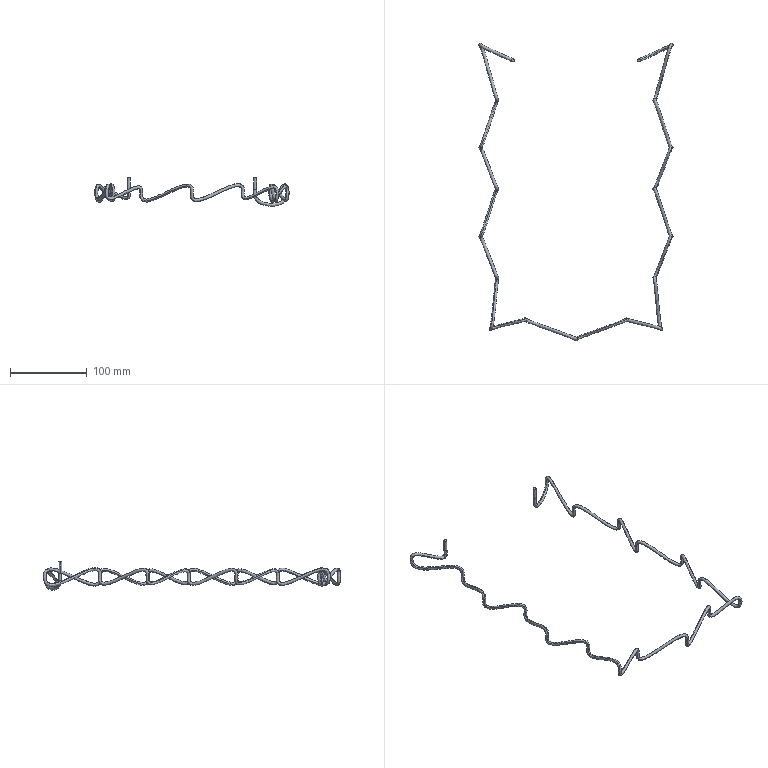Part | SolidWorks | features BaseBody 1 | 1 solid | 8 faces | box 252.714 x 386.443 x 36.966 mm | volume 28904 mm3 | cylinder 4 | spline 2 | plane 2 | commonest cylinder face diameters 4 x4